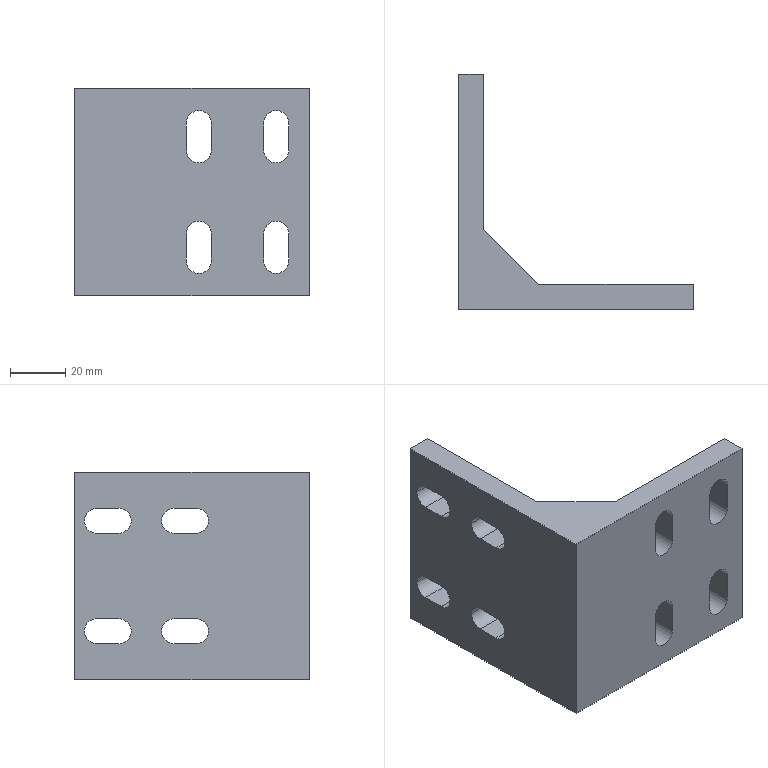Part | 1 solid | 45 faces | box 85 x 85 x 75 mm | volume 113263 mm3 | plane 25 | cylinder 20 | commonest cylinder face diameters 9 x20
STEP:
#1=CARTESIAN_POINT('',(0.,53.5,20.));
#2=VERTEX_POINT('',#1);
#3=CARTESIAN_POINT('',(0.,49.,24.5));
#4=VERTEX_POINT('',#3);
#5=CARTESIAN_POINT('',(0.,49.,20.));
#6=DIRECTION('',(1.,0.,0.));
#7=DIRECTION('',(0.,1.,0.));
#8=AXIS2_PLACEMENT_3D('',#5,#6,#7);
#9=CIRCLE('',#8,4.5);
#10=EDGE_CURVE('',#2,#4,#9,.T.);
#11=ORIENTED_EDGE('',*,*,#10,.F.);
#12=CARTESIAN_POINT('',(9.,53.5,20.));
#13=VERTEX_POINT('',#12);
#14=CARTESIAN_POINT('',(-66.,53.5,20.));
#15=DIRECTION('',(1.,0.,0.));
#16=VECTOR('',#15,1000.);
#17=LINE('',#14,#16);
#18=EDGE_CURVE('',#2,#13,#17,.T.);
#19=ORIENTED_EDGE('',*,*,#18,.T.);
#20=CARTESIAN_POINT('',(9.,49.,24.5));
#21=VERTEX_POINT('',#20);
#22=CARTESIAN_POINT('',(9.,49.,20.));
#23=DIRECTION('',(1.,0.,0.));
#24=DIRECTION('',(0.,-1.,0.));
#25=AXIS2_PLACEMENT_3D('',#22,#23,#24);
#26=CIRCLE('',#25,4.5);
#27=EDGE_CURVE('',#13,#21,#26,.T.);
#28=ORIENTED_EDGE('',*,*,#27,.T.);
#29=CARTESIAN_POINT('',(-66.,49.,24.5));
#30=DIRECTION('',(1.,0.,0.));
#31=VECTOR('',#30,1000.);
#32=LINE('',#29,#31);
#33=EDGE_CURVE('',#4,#21,#32,.T.);
#34=ORIENTED_EDGE('',*,*,#33,.F.);
#35=EDGE_LOOP('',(#11,#19,#28,#34));
#36=FACE_OUTER_BOUND('',#35,.T.);
#37=CARTESIAN_POINT('',(-66.,49.,20.));
#38=DIRECTION('',(1.,0.,0.));
#39=DIRECTION('',(0.,1.,0.));
#40=AXIS2_PLACEMENT_3D('',#37,#38,#39);
#41=CYLINDRICAL_SURFACE('',#40,4.5);
#42=ADVANCED_FACE('',(#36),#41,.F.);
#43=CARTESIAN_POINT('',(0.,53.5,-20.));
#44=VERTEX_POINT('',#43);
#45=CARTESIAN_POINT('',(0.,49.,-15.5));
#46=VERTEX_POINT('',#45);
#47=CARTESIAN_POINT('',(0.,49.,-20.));
#48=DIRECTION('',(1.,0.,0.));
#49=DIRECTION('',(0.,1.,0.));
#50=AXIS2_PLACEMENT_3D('',#47,#48,#49);
#51=CIRCLE('',#50,4.5);
#52=EDGE_CURVE('',#44,#46,#51,.T.);
#53=ORIENTED_EDGE('',*,*,#52,.F.);
#54=CARTESIAN_POINT('',(9.,53.5,-20.));
#55=VERTEX_POINT('',#54);
#56=CARTESIAN_POINT('',(-66.,53.5,-20.));
#57=DIRECTION('',(1.,0.,0.));
#58=VECTOR('',#57,1000.);
#59=LINE('',#56,#58);
#60=EDGE_CURVE('',#44,#55,#59,.T.);
#61=ORIENTED_EDGE('',*,*,#60,.T.);
#62=CARTESIAN_POINT('',(9.,49.,-15.5));
#63=VERTEX_POINT('',#62);
#64=CARTESIAN_POINT('',(9.,49.,-20.));
#65=DIRECTION('',(1.,0.,0.));
#66=DIRECTION('',(0.,1.,0.));
#67=AXIS2_PLACEMENT_3D('',#64,#65,#66);
#68=CIRCLE('',#67,4.5);
#69=EDGE_CURVE('',#55,#63,#68,.T.);
#70=ORIENTED_EDGE('',*,*,#69,.T.);
#71=CARTESIAN_POINT('',(-66.,49.,-15.5));
#72=DIRECTION('',(1.,0.,0.));
#73=VECTOR('',#72,1000.);
#74=LINE('',#71,#73);
#75=EDGE_CURVE('',#46,#63,#74,.T.);
#76=ORIENTED_EDGE('',*,*,#75,.F.);
#77=EDGE_LOOP('',(#53,#61,#70,#76));
#78=FACE_OUTER_BOUND('',#77,.T.);
#79=CARTESIAN_POINT('',(-66.,49.,-20.));
#80=DIRECTION('',(1.,0.,0.));
#81=DIRECTION('',(0.,1.,0.));
#82=AXIS2_PLACEMENT_3D('',#79,#80,#81);
#83=CYLINDRICAL_SURFACE('',#82,4.5);
#84=ADVANCED_FACE('',(#78),#83,.F.);
#85=CARTESIAN_POINT('',(0.,81.5,-20.));
#86=VERTEX_POINT('',#85);
#87=CARTESIAN_POINT('',(0.,77.,-15.5));
#88=VERTEX_POINT('',#87);
#89=CARTESIAN_POINT('',(0.,77.,-20.));
#90=DIRECTION('',(1.,0.,0.));
#91=DIRECTION('',(0.,1.,0.));
#92=AXIS2_PLACEMENT_3D('',#89,#90,#91);
#93=CIRCLE('',#92,4.5);
#94=EDGE_CURVE('',#86,#88,#93,.T.);
#95=ORIENTED_EDGE('',*,*,#94,.F.);
#96=CARTESIAN_POINT('',(9.,81.5,-20.));
#97=VERTEX_POINT('',#96);
#98=CARTESIAN_POINT('',(-66.,81.5,-20.));
#99=DIRECTION('',(1.,0.,0.));
#100=VECTOR('',#99,1000.);
#101=LINE('',#98,#100);
#102=EDGE_CURVE('',#86,#97,#101,.T.);
#103=ORIENTED_EDGE('',*,*,#102,.T.);
#104=CARTESIAN_POINT('',(9.,77.,-15.5));
#105=VERTEX_POINT('',#104);
#106=CARTESIAN_POINT('',(9.,77.,-20.));
#107=DIRECTION('',(1.,0.,0.));
#108=DIRECTION('',(0.,-1.,0.));
#109=AXIS2_PLACEMENT_3D('',#106,#107,#108);
#110=CIRCLE('',#109,4.5);
#111=EDGE_CURVE('',#97,#105,#110,.T.);
#112=ORIENTED_EDGE('',*,*,#111,.T.);
#113=CARTESIAN_POINT('',(-66.,77.,-15.5));
#114=DIRECTION('',(1.,0.,0.));
#115=VECTOR('',#114,1000.);
#116=LINE('',#113,#115);
#117=EDGE_CURVE('',#88,#105,#116,.T.);
#118=ORIENTED_EDGE('',*,*,#117,.F.);
#119=EDGE_LOOP('',(#95,#103,#112,#118));
#120=FACE_OUTER_BOUND('',#119,.T.);
#121=CARTESIAN_POINT('',(-66.,77.,-20.));
#122=DIRECTION('',(1.,0.,0.));
#123=DIRECTION('',(0.,1.,0.));
#124=AXIS2_PLACEMENT_3D('',#121,#122,#123);
#125=CYLINDRICAL_SURFACE('',#124,4.5);
#126=ADVANCED_FACE('',(#120),#125,.F.);
#127=CARTESIAN_POINT('',(0.,81.5,20.));
#128=VERTEX_POINT('',#127);
#129=CARTESIAN_POINT('',(0.,77.,24.5));
#130=VERTEX_POINT('',#129);
#131=CARTESIAN_POINT('',(0.,77.,20.));
#132=DIRECTION('',(1.,0.,0.));
#133=DIRECTION('',(0.,1.,0.));
#134=AXIS2_PLACEMENT_3D('',#131,#132,#133);
#135=CIRCLE('',#134,4.5);
#136=EDGE_CURVE('',#128,#130,#135,.T.);
#137=ORIENTED_EDGE('',*,*,#136,.F.);
#138=CARTESIAN_POINT('',(9.,81.5,20.));
#139=VERTEX_POINT('',#138);
#140=CARTESIAN_POINT('',(-66.,81.5,20.));
#141=DIRECTION('',(1.,0.,0.));
#142=VECTOR('',#141,1000.);
#143=LINE('',#140,#142);
#144=EDGE_CURVE('',#128,#139,#143,.T.);
#145=ORIENTED_EDGE('',*,*,#144,.T.);
#146=CARTESIAN_POINT('',(9.,77.,24.5));
#147=VERTEX_POINT('',#146);
#148=CARTESIAN_POINT('',(9.,77.,20.));
#149=DIRECTION('',(1.,0.,0.));
#150=DIRECTION('',(0.,1.,0.));
#151=AXIS2_PLACEMENT_3D('',#148,#149,#150);
#152=CIRCLE('',#151,4.5);
#153=EDGE_CURVE('',#139,#147,#152,.T.);
#154=ORIENTED_EDGE('',*,*,#153,.T.);
#155=CARTESIAN_POINT('',(-66.,77.,24.5));
#156=DIRECTION('',(1.,0.,0.));
#157=VECTOR('',#156,1000.);
#158=LINE('',#155,#157);
#159=EDGE_CURVE('',#130,#147,#158,.T.);
#160=ORIENTED_EDGE('',*,*,#159,.F.);
#161=EDGE_LOOP('',(#137,#145,#154,#160));
#162=FACE_OUTER_BOUND('',#161,.T.);
#163=CARTESIAN_POINT('',(-66.,77.,20.));
#164=DIRECTION('',(1.,0.,0.));
#165=DIRECTION('',(0.,1.,0.));
#166=AXIS2_PLACEMENT_3D('',#163,#164,#165);
#167=CYLINDRICAL_SURFACE('',#166,4.5);
#168=ADVANCED_FACE('',(#162),#167,.F.);
#169=CARTESIAN_POINT('',(0.,41.,24.5));
#170=VERTEX_POINT('',#169);
#171=CARTESIAN_POINT('',(0.,85.,24.5));
#172=DIRECTION('',(0.,-1.,0.));
#173=VECTOR('',#172,1000.);
#174=LINE('',#171,#173);
#175=EDGE_CURVE('',#4,#170,#174,.T.);
#176=ORIENTED_EDGE('',*,*,#175,.T.);
#177=CARTESIAN_POINT('',(0.,41.,15.5));
#178=VERTEX_POINT('',#177);
#179=CARTESIAN_POINT('',(0.,41.,20.));
#180=DIRECTION('',(1.,0.,0.));
#181=DIRECTION('',(0.,1.,0.));
#182=AXIS2_PLACEMENT_3D('',#179,#180,#181);
#183=CIRCLE('',#182,4.5);
#184=EDGE_CURVE('',#170,#178,#183,.T.);
#185=ORIENTED_EDGE('',*,*,#184,.T.);
#186=CARTESIAN_POINT('',(0.,49.,15.5));
#187=VERTEX_POINT('',#186);
#188=CARTESIAN_POINT('',(0.,85.,15.5));
#189=DIRECTION('',(0.,1.,0.));
#190=VECTOR('',#189,1000.);
#191=LINE('',#188,#190);
#192=EDGE_CURVE('',#178,#187,#191,.T.);
#193=ORIENTED_EDGE('',*,*,#192,.T.);
#194=CARTESIAN_POINT('',(0.,49.,20.));
#195=DIRECTION('',(1.,0.,0.));
#196=DIRECTION('',(0.,1.,0.));
#197=AXIS2_PLACEMENT_3D('',#194,#195,#196);
#198=CIRCLE('',#197,4.5);
#199=EDGE_CURVE('',#187,#2,#198,.T.);
#200=ORIENTED_EDGE('',*,*,#199,.T.);
#201=ORIENTED_EDGE('',*,*,#10,.T.);
#202=EDGE_LOOP('',(#176,#185,#193,#200,#201));
#203=FACE_BOUND('',#202,.T.);
#204=CARTESIAN_POINT('',(0.,41.,-15.5));
#205=VERTEX_POINT('',#204);
#206=CARTESIAN_POINT('',(0.,85.,-15.5));
#207=DIRECTION('',(0.,-1.,0.));
#208=VECTOR('',#207,1000.);
#209=LINE('',#206,#208);
#210=EDGE_CURVE('',#46,#205,#209,.T.);
#211=ORIENTED_EDGE('',*,*,#210,.T.);
#212=CARTESIAN_POINT('',(0.,41.,-24.5));
#213=VERTEX_POINT('',#212);
#214=CARTESIAN_POINT('',(0.,41.,-20.));
#215=DIRECTION('',(1.,0.,0.));
#216=DIRECTION('',(0.,1.,0.));
#217=AXIS2_PLACEMENT_3D('',#214,#215,#216);
#218=CIRCLE('',#217,4.5);
#219=EDGE_CURVE('',#205,#213,#218,.T.);
#220=ORIENTED_EDGE('',*,*,#219,.T.);
#221=CARTESIAN_POINT('',(0.,49.,-24.5));
#222=VERTEX_POINT('',#221);
#223=CARTESIAN_POINT('',(0.,85.,-24.5));
#224=DIRECTION('',(0.,1.,0.));
#225=VECTOR('',#224,1000.);
#226=LINE('',#223,#225);
#227=EDGE_CURVE('',#213,#222,#226,.T.);
#228=ORIENTED_EDGE('',*,*,#227,.T.);
#229=CARTESIAN_POINT('',(0.,49.,-20.));
#230=DIRECTION('',(1.,0.,0.));
#231=DIRECTION('',(0.,1.,0.));
#232=AXIS2_PLACEMENT_3D('',#229,#230,#231);
#233=CIRCLE('',#232,4.5);
#234=EDGE_CURVE('',#222,#44,#233,.T.);
#235=ORIENTED_EDGE('',*,*,#234,.T.);
#236=ORIENTED_EDGE('',*,*,#52,.T.);
#237=EDGE_LOOP('',(#211,#220,#228,#235,#236));
#238=FACE_BOUND('',#237,.T.);
#239=CARTESIAN_POINT('',(0.,69.,-24.5));
#240=VERTEX_POINT('',#239);
#241=CARTESIAN_POINT('',(0.,77.,-24.5));
#242=VERTEX_POINT('',#241);
#243=CARTESIAN_POINT('',(0.,85.,-24.5));
#244=DIRECTION('',(0.,1.,0.));
#245=VECTOR('',#244,1000.);
#246=LINE('',#243,#245);
#247=EDGE_CURVE('',#240,#242,#246,.T.);
#248=ORIENTED_EDGE('',*,*,#247,.T.);
#249=CARTESIAN_POINT('',(0.,77.,-20.));
#250=DIRECTION('',(1.,0.,0.));
#251=DIRECTION('',(0.,1.,0.));
#252=AXIS2_PLACEMENT_3D('',#249,#250,#251);
#253=CIRCLE('',#252,4.5);
#254=EDGE_CURVE('',#242,#86,#253,.T.);
#255=ORIENTED_EDGE('',*,*,#254,.T.);
#256=ORIENTED_EDGE('',*,*,#94,.T.);
#257=CARTESIAN_POINT('',(0.,69.,-15.5));
#258=VERTEX_POINT('',#257);
#259=CARTESIAN_POINT('',(0.,85.,-15.5));
#260=DIRECTION('',(0.,-1.,0.));
#261=VECTOR('',#260,1000.);
#262=LINE('',#259,#261);
#263=EDGE_CURVE('',#88,#258,#262,.T.);
#264=ORIENTED_EDGE('',*,*,#263,.T.);
#265=CARTESIAN_POINT('',(0.,69.,-20.));
#266=DIRECTION('',(1.,0.,0.));
#267=DIRECTION('',(0.,1.,0.));
#268=AXIS2_PLACEMENT_3D('',#265,#266,#267);
#269=CIRCLE('',#268,4.5);
#270=EDGE_CURVE('',#258,#240,#269,.T.);
#271=ORIENTED_EDGE('',*,*,#270,.T.);
#272=EDGE_LOOP('',(#248,#255,#256,#264,#271));
#273=FACE_BOUND('',#272,.T.);
#274=CARTESIAN_POINT('',(0.,69.,15.5));
#275=VERTEX_POINT('',#274);
#276=CARTESIAN_POINT('',(0.,77.,15.5));
#277=VERTEX_POINT('',#276);
#278=CARTESIAN_POINT('',(0.,85.,15.5));
#279=DIRECTION('',(0.,1.,0.));
#280=VECTOR('',#279,1000.);
#281=LINE('',#278,#280);
#282=EDGE_CURVE('',#275,#277,#281,.T.);
#283=ORIENTED_EDGE('',*,*,#282,.T.);
#284=CARTESIAN_POINT('',(0.,77.,20.));
#285=DIRECTION('',(1.,0.,0.));
#286=DIRECTION('',(0.,1.,0.));
#287=AXIS2_PLACEMENT_3D('',#284,#285,#286);
#288=CIRCLE('',#287,4.5);
#289=EDGE_CURVE('',#277,#128,#288,.T.);
#290=ORIENTED_EDGE('',*,*,#289,.T.);
#291=ORIENTED_EDGE('',*,*,#136,.T.);
#292=CARTESIAN_POINT('',(0.,69.,24.5));
#293=VERTEX_POINT('',#292);
#294=CARTESIAN_POINT('',(0.,85.,24.5));
#295=DIRECTION('',(0.,-1.,0.));
#296=VECTOR('',#295,1000.);
#297=LINE('',#294,#296);
#298=EDGE_CURVE('',#130,#293,#297,.T.);
#299=ORIENTED_EDGE('',*,*,#298,.T.);
#300=CARTESIAN_POINT('',(0.,69.,20.));
#301=DIRECTION('',(1.,0.,0.));
#302=DIRECTION('',(0.,1.,0.));
#303=AXIS2_PLACEMENT_3D('',#300,#301,#302);
#304=CIRCLE('',#303,4.5);
#305=EDGE_CURVE('',#293,#275,#304,.T.);
#306=ORIENTED_EDGE('',*,*,#305,.T.);
#307=EDGE_LOOP('',(#283,#290,#291,#299,#306));
#308=FACE_BOUND('',#307,.T.);
#309=CARTESIAN_POINT('',(0.,85.,-37.5));
#310=VERTEX_POINT('',#309);
#311=CARTESIAN_POINT('',(0.,0.,-37.5));
#312=VERTEX_POINT('',#311);
#313=CARTESIAN_POINT('',(0.,85.,-37.5));
#314=DIRECTION('',(0.,-1.,0.));
#315=VECTOR('',#314,1000.);
#316=LINE('',#313,#315);
#317=EDGE_CURVE('',#310,#312,#316,.T.);
#318=ORIENTED_EDGE('',*,*,#317,.T.);
#319=CARTESIAN_POINT('',(0.,0.,37.5));
#320=VERTEX_POINT('',#319);
#321=CARTESIAN_POINT('',(0.,0.,37.5));
#322=DIRECTION('',(0.,0.,-1.));
#323=VECTOR('',#322,1000.);
#324=LINE('',#321,#323);
#325=EDGE_CURVE('',#320,#312,#324,.T.);
#326=ORIENTED_EDGE('',*,*,#325,.F.);
#327=CARTESIAN_POINT('',(0.,85.,37.5));
#328=VERTEX_POINT('',#327);
#329=CARTESIAN_POINT('',(0.,85.,37.5));
#330=DIRECTION('',(0.,-1.,0.));
#331=VECTOR('',#330,1000.);
#332=LINE('',#329,#331);
#333=EDGE_CURVE('',#328,#320,#332,.T.);
#334=ORIENTED_EDGE('',*,*,#333,.F.);
#335=CARTESIAN_POINT('',(0.,85.,37.5));
#336=DIRECTION('',(0.,0.,-1.));
#337=VECTOR('',#336,1000.);
#338=LINE('',#335,#337);
#339=EDGE_CURVE('',#328,#310,#338,.T.);
#340=ORIENTED_EDGE('',*,*,#339,.T.);
#341=EDGE_LOOP('',(#318,#326,#334,#340));
#342=FACE_OUTER_BOUND('',#341,.T.);
#343=CARTESIAN_POINT('',(0.,85.,37.5));
#344=DIRECTION('',(1.,0.,0.));
#345=DIRECTION('',(0.,1.,0.));
#346=AXIS2_PLACEMENT_3D('',#343,#344,#345);
#347=PLANE('',#346);
#348=ADVANCED_FACE('',(#203,#238,#273,#308,#342),#347,.F.);
#349=CARTESIAN_POINT('',(68.5,0.,15.));
#350=VERTEX_POINT('',#349);
#351=CARTESIAN_POINT('',(68.5,0.,25.));
#352=VERTEX_POINT('',#351);
#353=CARTESIAN_POINT('',(68.5,0.,37.5));
#354=DIRECTION('',(0.,0.,1.));
#355=VECTOR('',#354,1000.);
#356=LINE('',#353,#355);
#357=EDGE_CURVE('',#350,#352,#356,.T.);
#358=ORIENTED_EDGE('',*,*,#357,.T.);
#359=CARTESIAN_POINT('',(77.5,0.,25.));
#360=VERTEX_POINT('',#359);
#361=CARTESIAN_POINT('',(73.,0.,25.));
#362=DIRECTION('',(0.,1.,0.));
#363=DIRECTION('',(0.,0.,1.));
#364=AXIS2_PLACEMENT_3D('',#361,#362,#363);
#365=CIRCLE('',#364,4.5);
#366=EDGE_CURVE('',#352,#360,#365,.T.);
#367=ORIENTED_EDGE('',*,*,#366,.T.);
#368=CARTESIAN_POINT('',(77.5,0.,15.));
#369=VERTEX_POINT('',#368);
#370=CARTESIAN_POINT('',(77.5,0.,37.5));
#371=DIRECTION('',(0.,0.,-1.));
#372=VECTOR('',#371,1000.);
#373=LINE('',#370,#372);
#374=EDGE_CURVE('',#360,#369,#373,.T.);
#375=ORIENTED_EDGE('',*,*,#374,.T.);
#376=CARTESIAN_POINT('',(73.,0.,15.));
#377=DIRECTION('',(0.,1.,0.));
#378=DIRECTION('',(0.,0.,1.));
#379=AXIS2_PLACEMENT_3D('',#376,#377,#378);
#380=CIRCLE('',#379,4.5);
#381=EDGE_CURVE('',#369,#350,#380,.T.);
#382=ORIENTED_EDGE('',*,*,#381,.T.);
#383=EDGE_LOOP('',(#358,#367,#375,#382));
#384=FACE_BOUND('',#383,.T.);
#385=CARTESIAN_POINT('',(40.5,0.,15.));
#386=VERTEX_POINT('',#385);
#387=CARTESIAN_POINT('',(40.5,0.,25.));
#388=VERTEX_POINT('',#387);
#389=CARTESIAN_POINT('',(40.5,0.,37.5));
#390=DIRECTION('',(0.,0.,1.));
#391=VECTOR('',#390,1000.);
#392=LINE('',#389,#391);
#393=EDGE_CURVE('',#386,#388,#392,.T.);
#394=ORIENTED_EDGE('',*,*,#393,.T.);
#395=CARTESIAN_POINT('',(49.5,0.,25.));
#396=VERTEX_POINT('',#395);
#397=CARTESIAN_POINT('',(45.,0.,25.));
#398=DIRECTION('',(0.,1.,0.));
#399=DIRECTION('',(0.,0.,1.));
#400=AXIS2_PLACEMENT_3D('',#397,#398,#399);
#401=CIRCLE('',#400,4.5);
#402=EDGE_CURVE('',#388,#396,#401,.T.);
#403=ORIENTED_EDGE('',*,*,#402,.T.);
#404=CARTESIAN_POINT('',(49.5,0.,15.));
#405=VERTEX_POINT('',#404);
#406=CARTESIAN_POINT('',(49.5,0.,37.5));
#407=DIRECTION('',(0.,0.,-1.));
#408=VECTOR('',#407,1000.);
#409=LINE('',#406,#408);
#410=EDGE_CURVE('',#396,#405,#409,.T.);
#411=ORIENTED_EDGE('',*,*,#410,.T.);
#412=CARTESIAN_POINT('',(45.,0.,15.));
#413=DIRECTION('',(0.,1.,0.));
#414=DIRECTION('',(0.,0.,1.));
#415=AXIS2_PLACEMENT_3D('',#412,#413,#414);
#416=CIRCLE('',#415,4.5);
#417=EDGE_CURVE('',#405,#386,#416,.T.);
#418=ORIENTED_EDGE('',*,*,#417,.T.);
#419=EDGE_LOOP('',(#394,#403,#411,#418));
#420=FACE_BOUND('',#419,.T.);
#421=CARTESIAN_POINT('',(68.5,0.,-25.));
#422=VERTEX_POINT('',#421);
#423=CARTESIAN_POINT('',(68.5,0.,-15.));
#424=VERTEX_POINT('',#423);
#425=CARTESIAN_POINT('',(68.5,0.,37.5));
#426=DIRECTION('',(0.,0.,1.));
#427=VECTOR('',#426,1000.);
#428=LINE('',#425,#427);
#429=EDGE_CURVE('',#422,#424,#428,.T.);
#430=ORIENTED_EDGE('',*,*,#429,.T.);
#431=CARTESIAN_POINT('',(77.5,0.,-15.));
#432=VERTEX_POINT('',#431);
#433=CARTESIAN_POINT('',(73.,0.,-15.));
#434=DIRECTION('',(0.,1.,0.));
#435=DIRECTION('',(0.,0.,1.));
#436=AXIS2_PLACEMENT_3D('',#433,#434,#435);
#437=CIRCLE('',#436,4.5);
#438=EDGE_CURVE('',#424,#432,#437,.T.);
#439=ORIENTED_EDGE('',*,*,#438,.T.);
#440=CARTESIAN_POINT('',(77.5,0.,-25.));
#441=VERTEX_POINT('',#440);
#442=CARTESIAN_POINT('',(77.5,0.,37.5));
#443=DIRECTION('',(0.,0.,-1.));
#444=VECTOR('',#443,1000.);
#445=LINE('',#442,#444);
#446=EDGE_CURVE('',#432,#441,#445,.T.);
#447=ORIENTED_EDGE('',*,*,#446,.T.);
#448=CARTESIAN_POINT('',(73.,0.,-25.));
#449=DIRECTION('',(0.,1.,0.));
#450=DIRECTION('',(0.,0.,1.));
#451=AXIS2_PLACEMENT_3D('',#448,#449,#450);
#452=CIRCLE('',#451,4.5);
#453=EDGE_CURVE('',#441,#422,#452,.T.);
#454=ORIENTED_EDGE('',*,*,#453,.T.);
#455=EDGE_LOOP('',(#430,#439,#447,#454));
#456=FACE_BOUND('',#455,.T.);
#457=CARTESIAN_POINT('',(40.5,0.,-25.));
#458=VERTEX_POINT('',#457);
#459=CARTESIAN_POINT('',(40.5,0.,-15.));
#460=VERTEX_POINT('',#459);
#461=CARTESIAN_POINT('',(40.5,0.,37.5));
#462=DIRECTION('',(0.,0.,1.));
#463=VECTOR('',#462,1000.);
#464=LINE('',#461,#463);
#465=EDGE_CURVE('',#458,#460,#464,.T.);
#466=ORIENTED_EDGE('',*,*,#465,.T.);
#467=CARTESIAN_POINT('',(49.5,0.,-15.));
#468=VERTEX_POINT('',#467);
#469=CARTESIAN_POINT('',(45.,0.,-15.));
#470=DIRECTION('',(0.,1.,0.));
#471=DIRECTION('',(0.,0.,1.));
#472=AXIS2_PLACEMENT_3D('',#469,#470,#471);
#473=CIRCLE('',#472,4.5);
#474=EDGE_CURVE('',#460,#468,#473,.T.);
#475=ORIENTED_EDGE('',*,*,#474,.T.);
#476=CARTESIAN_POINT('',(49.5,0.,-25.));
#477=VERTEX_POINT('',#476);
#478=CARTESIAN_POINT('',(49.5,0.,37.5));
#479=DIRECTION('',(0.,0.,-1.));
#480=VECTOR('',#479,1000.);
#481=LINE('',#478,#480);
#482=EDGE_CURVE('',#468,#477,#481,.T.);
#483=ORIENTED_EDGE('',*,*,#482,.T.);
#484=CARTESIAN_POINT('',(45.,0.,-25.));
#485=DIRECTION('',(0.,1.,0.));
#486=DIRECTION('',(0.,0.,1.));
#487=AXIS2_PLACEMENT_3D('',#484,#485,#486);
#488=CIRCLE('',#487,4.5);
#489=EDGE_CURVE('',#477,#458,#488,.T.);
#490=ORIENTED_EDGE('',*,*,#489,.T.);
#491=EDGE_LOOP('',(#466,#475,#483,#490));
#492=FACE_BOUND('',#491,.T.);
#493=CARTESIAN_POINT('',(85.,0.,-37.5));
#494=VERTEX_POINT('',#493);
#495=CARTESIAN_POINT('',(0.,0.,-37.5));
#496=DIRECTION('',(1.,0.,0.));
#497=VECTOR('',#496,1000.);
#498=LINE('',#495,#497);
#499=EDGE_CURVE('',#312,#494,#498,.T.);
#500=ORIENTED_EDGE('',*,*,#499,.T.);
#501=CARTESIAN_POINT('',(85.,0.,37.5));
#502=VERTEX_POINT('',#501);
#503=CARTESIAN_POINT('',(85.,0.,37.5));
#504=DIRECTION('',(0.,0.,-1.));
#505=VECTOR('',#504,1000.);
#506=LINE('',#503,#505);
#507=EDGE_CURVE('',#502,#494,#506,.T.);
#508=ORIENTED_EDGE('',*,*,#507,.F.);
#509=CARTESIAN_POINT('',(0.,0.,37.5));
#510=DIRECTION('',(1.,0.,0.));
#511=VECTOR('',#510,1000.);
#512=LINE('',#509,#511);
#513=EDGE_CURVE('',#320,#502,#512,.T.);
#514=ORIENTED_EDGE('',*,*,#513,.F.);
#515=ORIENTED_EDGE('',*,*,#325,.T.);
#516=EDGE_LOOP('',(#500,#508,#514,#515));
#517=FACE_OUTER_BOUND('',#516,.T.);
#518=CARTESIAN_POINT('',(0.,0.,37.5));
#519=DIRECTION('',(0.,1.,0.));
#520=DIRECTION('',(0.,0.,1.));
#521=AXIS2_PLACEMENT_3D('',#518,#519,#520);
#522=PLANE('',#521);
#523=ADVANCED_FACE('',(#384,#420,#456,#492,#517),#522,.F.);
#524=CARTESIAN_POINT('',(85.,9.,-37.5));
#525=VERTEX_POINT('',#524);
#526=CARTESIAN_POINT('',(85.,0.,-37.5));
#527=DIRECTION('',(0.,1.,0.));
#528=VECTOR('',#527,1000.);
#529=LINE('',#526,#528);
#530=EDGE_CURVE('',#494,#525,#529,.T.);
#531=ORIENTED_EDGE('',*,*,#530,.T.);
#532=CARTESIAN_POINT('',(85.,9.,37.5));
#533=VERTEX_POINT('',#532);
#534=CARTESIAN_POINT('',(85.,9.,37.5));
#535=DIRECTION('',(0.,0.,-1.));
#536=VECTOR('',#535,1000.);
#537=LINE('',#534,#536);
#538=EDGE_CURVE('',#533,#525,#537,.T.);
#539=ORIENTED_EDGE('',*,*,#538,.F.);
#540=CARTESIAN_POINT('',(85.,0.,37.5));
#541=DIRECTION('',(0.,1.,0.));
#542=VECTOR('',#541,1000.);
#543=LINE('',#540,#542);
#544=EDGE_CURVE('',#502,#533,#543,.T.);
#545=ORIENTED_EDGE('',*,*,#544,.F.);
#546=ORIENTED_EDGE('',*,*,#507,.T.);
#547=EDGE_LOOP('',(#531,#539,#545,#546));
#548=FACE_OUTER_BOUND('',#547,.T.);
#549=CARTESIAN_POINT('',(85.,0.,37.5));
#550=DIRECTION('',(-1.,0.,0.));
#551=DIRECTION('',(0.,0.,1.));
#552=AXIS2_PLACEMENT_3D('',#549,#550,#551);
#553=PLANE('',#552);
#554=ADVANCED_FACE('',(#548),#553,.F.);
#555=CARTESIAN_POINT('',(77.5,9.,25.));
#556=VERTEX_POINT('',#555);
#557=CARTESIAN_POINT('',(77.5,9.,15.));
#558=VERTEX_POINT('',#557);
#559=CARTESIAN_POINT('',(77.5,9.,25.));
#560=DIRECTION('',(0.,0.,-1.));
#561=VECTOR('',#560,1000.);
#562=LINE('',#559,#561);
#563=EDGE_CURVE('',#556,#558,#562,.T.);
#564=ORIENTED_EDGE('',*,*,#563,.F.);
#565=CARTESIAN_POINT('',(68.5,9.,25.));
#566=VERTEX_POINT('',#565);
#567=CARTESIAN_POINT('',(73.,9.,25.));
#568=DIRECTION('',(0.,1.,0.));
#569=DIRECTION('',(-1.,0.,0.));
#570=AXIS2_PLACEMENT_3D('',#567,#568,#569);
#571=CIRCLE('',#570,4.5);
#572=EDGE_CURVE('',#566,#556,#571,.T.);
#573=ORIENTED_EDGE('',*,*,#572,.F.);
#574=CARTESIAN_POINT('',(68.5,9.,15.));
#575=VERTEX_POINT('',#574);
#576=CARTESIAN_POINT('',(68.5,9.,25.));
#577=DIRECTION('',(0.,0.,1.));
#578=VECTOR('',#577,1000.);
#579=LINE('',#576,#578);
#580=EDGE_CURVE('',#575,#566,#579,.T.);
#581=ORIENTED_EDGE('',*,*,#580,.F.);
#582=CARTESIAN_POINT('',(73.,9.,15.));
#583=DIRECTION('',(0.,1.,0.));
#584=DIRECTION('',(-1.,0.,0.));
#585=AXIS2_PLACEMENT_3D('',#582,#583,#584);
#586=CIRCLE('',#585,4.5);
#587=EDGE_CURVE('',#558,#575,#586,.T.);
#588=ORIENTED_EDGE('',*,*,#587,.F.);
#589=EDGE_LOOP('',(#564,#573,#581,#588));
#590=FACE_BOUND('',#589,.T.);
#591=CARTESIAN_POINT('',(49.5,9.,25.));
#592=VERTEX_POINT('',#591);
#593=CARTESIAN_POINT('',(49.5,9.,15.));
#594=VERTEX_POINT('',#593);
#595=CARTESIAN_POINT('',(49.5,9.,25.));
#596=DIRECTION('',(0.,0.,-1.));
#597=VECTOR('',#596,1000.);
#598=LINE('',#595,#597);
#599=EDGE_CURVE('',#592,#594,#598,.T.);
#600=ORIENTED_EDGE('',*,*,#599,.F.);
#601=CARTESIAN_POINT('',(40.5,9.,25.));
#602=VERTEX_POINT('',#601);
#603=CARTESIAN_POINT('',(45.,9.,25.));
#604=DIRECTION('',(0.,1.,0.));
#605=DIRECTION('',(-1.,0.,0.));
#606=AXIS2_PLACEMENT_3D('',#603,#604,#605);
#607=CIRCLE('',#606,4.5);
#608=EDGE_CURVE('',#602,#592,#607,.T.);
#609=ORIENTED_EDGE('',*,*,#608,.F.);
#610=CARTESIAN_POINT('',(40.5,9.,15.));
#611=VERTEX_POINT('',#610);
#612=CARTESIAN_POINT('',(40.5,9.,25.));
#613=DIRECTION('',(0.,0.,1.));
#614=VECTOR('',#613,1000.);
#615=LINE('',#612,#614);
#616=EDGE_CURVE('',#611,#602,#615,.T.);
#617=ORIENTED_EDGE('',*,*,#616,.F.);
#618=CARTESIAN_POINT('',(45.,9.,15.));
#619=DIRECTION('',(0.,1.,0.));
#620=DIRECTION('',(-1.,0.,0.));
#621=AXIS2_PLACEMENT_3D('',#618,#619,#620);
#622=CIRCLE('',#621,4.5);
#623=EDGE_CURVE('',#594,#611,#622,.T.);
#624=ORIENTED_EDGE('',*,*,#623,.F.);
#625=EDGE_LOOP('',(#600,#609,#617,#624));
#626=FACE_BOUND('',#625,.T.);
#627=CARTESIAN_POINT('',(77.5,9.,-15.));
#628=VERTEX_POINT('',#627);
#629=CARTESIAN_POINT('',(77.5,9.,-25.));
#630=VERTEX_POINT('',#629);
#631=CARTESIAN_POINT('',(77.5,9.,-15.));
#632=DIRECTION('',(0.,0.,-1.));
#633=VECTOR('',#632,1000.);
#634=LINE('',#631,#633);
#635=EDGE_CURVE('',#628,#630,#634,.T.);
#636=ORIENTED_EDGE('',*,*,#635,.F.);
#637=CARTESIAN_POINT('',(68.5,9.,-15.));
#638=VERTEX_POINT('',#637);
#639=CARTESIAN_POINT('',(73.,9.,-15.));
#640=DIRECTION('',(0.,1.,0.));
#641=DIRECTION('',(-1.,0.,0.));
#642=AXIS2_PLACEMENT_3D('',#639,#640,#641);
#643=CIRCLE('',#642,4.5);
#644=EDGE_CURVE('',#638,#628,#643,.T.);
#645=ORIENTED_EDGE('',*,*,#644,.F.);
#646=CARTESIAN_POINT('',(68.5,9.,-25.));
#647=VERTEX_POINT('',#646);
#648=CARTESIAN_POINT('',(68.5,9.,-15.));
#649=DIRECTION('',(0.,0.,1.));
#650=VECTOR('',#649,1000.);
#651=LINE('',#648,#650);
#652=EDGE_CURVE('',#647,#638,#651,.T.);
#653=ORIENTED_EDGE('',*,*,#652,.F.);
#654=CARTESIAN_POINT('',(73.,9.,-25.));
#655=DIRECTION('',(0.,1.,0.));
#656=DIRECTION('',(-1.,0.,0.));
#657=AXIS2_PLACEMENT_3D('',#654,#655,#656);
#658=CIRCLE('',#657,4.5);
#659=EDGE_CURVE('',#630,#647,#658,.T.);
#660=ORIENTED_EDGE('',*,*,#659,.F.);
#661=EDGE_LOOP('',(#636,#645,#653,#660));
#662=FACE_BOUND('',#661,.T.);
#663=CARTESIAN_POINT('',(49.5,9.,-15.));
#664=VERTEX_POINT('',#663);
#665=CARTESIAN_POINT('',(49.5,9.,-25.));
#666=VERTEX_POINT('',#665);
#667=CARTESIAN_POINT('',(49.5,9.,-15.));
#668=DIRECTION('',(0.,0.,-1.));
#669=VECTOR('',#668,1000.);
#670=LINE('',#667,#669);
#671=EDGE_CURVE('',#664,#666,#670,.T.);
#672=ORIENTED_EDGE('',*,*,#671,.F.);
#673=CARTESIAN_POINT('',(40.5,9.,-15.));
#674=VERTEX_POINT('',#673);
#675=CARTESIAN_POINT('',(45.,9.,-15.));
#676=DIRECTION('',(0.,1.,0.));
#677=DIRECTION('',(-1.,0.,0.));
#678=AXIS2_PLACEMENT_3D('',#675,#676,#677);
#679=CIRCLE('',#678,4.5);
#680=EDGE_CURVE('',#674,#664,#679,.T.);
#681=ORIENTED_EDGE('',*,*,#680,.F.);
#682=CARTESIAN_POINT('',(40.5,9.,-25.));
#683=VERTEX_POINT('',#682);
#684=CARTESIAN_POINT('',(40.5,9.,-15.));
#685=DIRECTION('',(0.,0.,1.));
#686=VECTOR('',#685,1000.);
#687=LINE('',#684,#686);
#688=EDGE_CURVE('',#683,#674,#687,.T.);
#689=ORIENTED_EDGE('',*,*,#688,.F.);
#690=CARTESIAN_POINT('',(45.,9.,-25.));
#691=DIRECTION('',(0.,1.,0.));
#692=DIRECTION('',(-1.,0.,0.));
#693=AXIS2_PLACEMENT_3D('',#690,#691,#692);
#694=CIRCLE('',#693,4.5);
#695=EDGE_CURVE('',#666,#683,#694,.T.);
#696=ORIENTED_EDGE('',*,*,#695,.F.);
#697=EDGE_LOOP('',(#672,#681,#689,#696));
#698=FACE_BOUND('',#697,.T.);
#699=CARTESIAN_POINT('',(29.,9.,-37.5));
#700=VERTEX_POINT('',#699);
#701=CARTESIAN_POINT('',(85.,9.,-37.5));
#702=DIRECTION('',(-1.,0.,0.));
#703=VECTOR('',#702,1000.);
#704=LINE('',#701,#703);
#705=EDGE_CURVE('',#525,#700,#704,.T.);
#706=ORIENTED_EDGE('',*,*,#705,.T.);
#707=CARTESIAN_POINT('',(29.,9.,37.5));
#708=VERTEX_POINT('',#707);
#709=CARTESIAN_POINT('',(29.,9.,37.5));
#710=DIRECTION('',(0.,0.,-1.));
#711=VECTOR('',#710,1000.);
#712=LINE('',#709,#711);
#713=EDGE_CURVE('',#708,#700,#712,.T.);
#714=ORIENTED_EDGE('',*,*,#713,.F.);
#715=CARTESIAN_POINT('',(85.,9.,37.5));
#716=DIRECTION('',(-1.,0.,0.));
#717=VECTOR('',#716,1000.);
#718=LINE('',#715,#717);
#719=EDGE_CURVE('',#533,#708,#718,.T.);
#720=ORIENTED_EDGE('',*,*,#719,.F.);
#721=ORIENTED_EDGE('',*,*,#538,.T.);
#722=EDGE_LOOP('',(#706,#714,#720,#721));
#723=FACE_OUTER_BOUND('',#722,.T.);
#724=CARTESIAN_POINT('',(85.,9.,37.5));
#725=DIRECTION('',(0.,-1.,0.));
#726=DIRECTION('',(1.,0.,0.));
#727=AXIS2_PLACEMENT_3D('',#724,#725,#726);
#728=PLANE('',#727);
#729=ADVANCED_FACE('',(#590,#626,#662,#698,#723),#728,.F.);
#730=CARTESIAN_POINT('',(9.,29.,-37.5));
#731=VERTEX_POINT('',#730);
#732=CARTESIAN_POINT('',(9.,29.,-37.5));
#733=DIRECTION('',(-0.7071,0.7071,0.));
#734=VECTOR('',#733,1000.);
#735=LINE('',#732,#734);
#736=EDGE_CURVE('',#700,#731,#735,.T.);
#737=ORIENTED_EDGE('',*,*,#736,.T.);
#738=CARTESIAN_POINT('',(9.,29.,37.5));
#739=VERTEX_POINT('',#738);
#740=CARTESIAN_POINT('',(9.,29.,37.5));
#741=DIRECTION('',(0.,0.,-1.));
#742=VECTOR('',#741,1000.);
#743=LINE('',#740,#742);
#744=EDGE_CURVE('',#739,#731,#743,.T.);
#745=ORIENTED_EDGE('',*,*,#744,.F.);
#746=CARTESIAN_POINT('',(9.,29.,37.5));
#747=DIRECTION('',(-0.7071,0.7071,0.));
#748=VECTOR('',#747,1000.);
#749=LINE('',#746,#748);
#750=EDGE_CURVE('',#708,#739,#749,.T.);
#751=ORIENTED_EDGE('',*,*,#750,.F.);
#752=ORIENTED_EDGE('',*,*,#713,.T.);
#753=EDGE_LOOP('',(#737,#745,#751,#752));
#754=FACE_OUTER_BOUND('',#753,.T.);
#755=CARTESIAN_POINT('',(9.,29.,37.5));
#756=DIRECTION('',(-0.7071,-0.7071,0.));
#757=DIRECTION('',(0.7071,-0.7071,0.));
#758=AXIS2_PLACEMENT_3D('',#755,#756,#757);
#759=PLANE('',#758);
#760=ADVANCED_FACE('',(#754),#759,.F.);
#761=CARTESIAN_POINT('',(9.,41.,15.5));
#762=VERTEX_POINT('',#761);
#763=CARTESIAN_POINT('',(9.,49.,15.5));
#764=VERTEX_POINT('',#763);
#765=CARTESIAN_POINT('',(9.,41.,15.5));
#766=DIRECTION('',(0.,1.,0.));
#767=VECTOR('',#766,1000.);
#768=LINE('',#765,#767);
#769=EDGE_CURVE('',#762,#764,#768,.T.);
#770=ORIENTED_EDGE('',*,*,#769,.F.);
#771=CARTESIAN_POINT('',(9.,41.,24.5));
#772=VERTEX_POINT('',#771);
#773=CARTESIAN_POINT('',(9.,41.,20.));
#774=DIRECTION('',(1.,0.,0.));
#775=DIRECTION('',(0.,-1.,0.));
#776=AXIS2_PLACEMENT_3D('',#773,#774,#775);
#777=CIRCLE('',#776,4.5);
#778=EDGE_CURVE('',#772,#762,#777,.T.);
#779=ORIENTED_EDGE('',*,*,#778,.F.);
#780=CARTESIAN_POINT('',(9.,41.,24.5));
#781=DIRECTION('',(0.,-1.,0.));
#782=VECTOR('',#781,1000.);
#783=LINE('',#780,#782);
#784=EDGE_CURVE('',#21,#772,#783,.T.);
#785=ORIENTED_EDGE('',*,*,#784,.F.);
#786=ORIENTED_EDGE('',*,*,#27,.F.);
#787=CARTESIAN_POINT('',(9.,49.,20.));
#788=DIRECTION('',(1.,0.,0.));
#789=DIRECTION('',(0.,-1.,0.));
#790=AXIS2_PLACEMENT_3D('',#787,#788,#789);
#791=CIRCLE('',#790,4.5);
#792=EDGE_CURVE('',#764,#13,#791,.T.);
#793=ORIENTED_EDGE('',*,*,#792,.F.);
#794=EDGE_LOOP('',(#770,#779,#785,#786,#793));
#795=FACE_BOUND('',#794,.T.);
#796=CARTESIAN_POINT('',(9.,41.,-24.5));
#797=VERTEX_POINT('',#796);
#798=CARTESIAN_POINT('',(9.,49.,-24.5));
#799=VERTEX_POINT('',#798);
#800=CARTESIAN_POINT('',(9.,41.,-24.5));
#801=DIRECTION('',(0.,1.,0.));
#802=VECTOR('',#801,1000.);
#803=LINE('',#800,#802);
#804=EDGE_CURVE('',#797,#799,#803,.T.);
#805=ORIENTED_EDGE('',*,*,#804,.F.);
#806=CARTESIAN_POINT('',(9.,41.,-15.5));
#807=VERTEX_POINT('',#806);
#808=CARTESIAN_POINT('',(9.,41.,-20.));
#809=DIRECTION('',(1.,0.,0.));
#810=DIRECTION('',(0.,1.,0.));
#811=AXIS2_PLACEMENT_3D('',#808,#809,#810);
#812=CIRCLE('',#811,4.5);
#813=EDGE_CURVE('',#807,#797,#812,.T.);
#814=ORIENTED_EDGE('',*,*,#813,.F.);
#815=CARTESIAN_POINT('',(9.,41.,-15.5));
#816=DIRECTION('',(0.,-1.,0.));
#817=VECTOR('',#816,1000.);
#818=LINE('',#815,#817);
#819=EDGE_CURVE('',#63,#807,#818,.T.);
#820=ORIENTED_EDGE('',*,*,#819,.F.);
#821=ORIENTED_EDGE('',*,*,#69,.F.);
#822=CARTESIAN_POINT('',(9.,49.,-20.));
#823=DIRECTION('',(1.,0.,0.));
#824=DIRECTION('',(0.,1.,0.));
#825=AXIS2_PLACEMENT_3D('',#822,#823,#824);
#826=CIRCLE('',#825,4.5);
#827=EDGE_CURVE('',#799,#55,#826,.T.);
#828=ORIENTED_EDGE('',*,*,#827,.F.);
#829=EDGE_LOOP('',(#805,#814,#820,#821,#828));
#830=FACE_BOUND('',#829,.T.);
#831=CARTESIAN_POINT('',(9.,69.,-15.5));
#832=VERTEX_POINT('',#831);
#833=CARTESIAN_POINT('',(9.,77.,-15.5));
#834=DIRECTION('',(0.,-1.,0.));
#835=VECTOR('',#834,1000.);
#836=LINE('',#833,#835);
#837=EDGE_CURVE('',#105,#832,#836,.T.);
#838=ORIENTED_EDGE('',*,*,#837,.F.);
#839=ORIENTED_EDGE('',*,*,#111,.F.);
#840=CARTESIAN_POINT('',(9.,77.,-24.5));
#841=VERTEX_POINT('',#840);
#842=CARTESIAN_POINT('',(9.,77.,-20.));
#843=DIRECTION('',(1.,0.,0.));
#844=DIRECTION('',(0.,-1.,0.));
#845=AXIS2_PLACEMENT_3D('',#842,#843,#844);
#846=CIRCLE('',#845,4.5);
#847=EDGE_CURVE('',#841,#97,#846,.T.);
#848=ORIENTED_EDGE('',*,*,#847,.F.);
#849=CARTESIAN_POINT('',(9.,69.,-24.5));
#850=VERTEX_POINT('',#849);
#851=CARTESIAN_POINT('',(9.,77.,-24.5));
#852=DIRECTION('',(0.,1.,0.));
#853=VECTOR('',#852,1000.);
#854=LINE('',#851,#853);
#855=EDGE_CURVE('',#850,#841,#854,.T.);
#856=ORIENTED_EDGE('',*,*,#855,.F.);
#857=CARTESIAN_POINT('',(9.,69.,-20.));
#858=DIRECTION('',(1.,0.,0.));
#859=DIRECTION('',(0.,-1.,0.));
#860=AXIS2_PLACEMENT_3D('',#857,#858,#859);
#861=CIRCLE('',#860,4.5);
#862=EDGE_CURVE('',#832,#850,#861,.T.);
#863=ORIENTED_EDGE('',*,*,#862,.F.);
#864=EDGE_LOOP('',(#838,#839,#848,#856,#863));
#865=FACE_BOUND('',#864,.T.);
#866=CARTESIAN_POINT('',(9.,69.,24.5));
#867=VERTEX_POINT('',#866);
#868=CARTESIAN_POINT('',(9.,77.,24.5));
#869=DIRECTION('',(0.,-1.,0.));
#870=VECTOR('',#869,1000.);
#871=LINE('',#868,#870);
#872=EDGE_CURVE('',#147,#867,#871,.T.);
#873=ORIENTED_EDGE('',*,*,#872,.F.);
#874=ORIENTED_EDGE('',*,*,#153,.F.);
#875=CARTESIAN_POINT('',(9.,77.,15.5));
#876=VERTEX_POINT('',#875);
#877=CARTESIAN_POINT('',(9.,77.,20.));
#878=DIRECTION('',(1.,0.,0.));
#879=DIRECTION('',(0.,1.,0.));
#880=AXIS2_PLACEMENT_3D('',#877,#878,#879);
#881=CIRCLE('',#880,4.5);
#882=EDGE_CURVE('',#876,#139,#881,.T.);
#883=ORIENTED_EDGE('',*,*,#882,.F.);
#884=CARTESIAN_POINT('',(9.,69.,15.5));
#885=VERTEX_POINT('',#884);
#886=CARTESIAN_POINT('',(9.,77.,15.5));
#887=DIRECTION('',(0.,1.,0.));
#888=VECTOR('',#887,1000.);
#889=LINE('',#886,#888);
#890=EDGE_CURVE('',#885,#876,#889,.T.);
#891=ORIENTED_EDGE('',*,*,#890,.F.);
#892=CARTESIAN_POINT('',(9.,69.,20.));
#893=DIRECTION('',(1.,0.,0.));
#894=DIRECTION('',(0.,1.,0.));
#895=AXIS2_PLACEMENT_3D('',#892,#893,#894);
#896=CIRCLE('',#895,4.5);
#897=EDGE_CURVE('',#867,#885,#896,.T.);
#898=ORIENTED_EDGE('',*,*,#897,.F.);
#899=EDGE_LOOP('',(#873,#874,#883,#891,#898));
#900=FACE_BOUND('',#899,.T.);
#901=CARTESIAN_POINT('',(9.,85.,-37.5));
#902=VERTEX_POINT('',#901);
#903=CARTESIAN_POINT('',(9.,29.,-37.5));
#904=DIRECTION('',(0.,1.,0.));
#905=VECTOR('',#904,1000.);
#906=LINE('',#903,#905);
#907=EDGE_CURVE('',#731,#902,#906,.T.);
#908=ORIENTED_EDGE('',*,*,#907,.T.);
#909=CARTESIAN_POINT('',(9.,85.,37.5));
#910=VERTEX_POINT('',#909);
#911=CARTESIAN_POINT('',(9.,85.,37.5));
#912=DIRECTION('',(0.,0.,-1.));
#913=VECTOR('',#912,1000.);
#914=LINE('',#911,#913);
#915=EDGE_CURVE('',#910,#902,#914,.T.);
#916=ORIENTED_EDGE('',*,*,#915,.F.);
#917=CARTESIAN_POINT('',(9.,29.,37.5));
#918=DIRECTION('',(0.,1.,0.));
#919=VECTOR('',#918,1000.);
#920=LINE('',#917,#919);
#921=EDGE_CURVE('',#739,#910,#920,.T.);
#922=ORIENTED_EDGE('',*,*,#921,.F.);
#923=ORIENTED_EDGE('',*,*,#744,.T.);
#924=EDGE_LOOP('',(#908,#916,#922,#923));
#925=FACE_OUTER_BOUND('',#924,.T.);
#926=CARTESIAN_POINT('',(9.,29.,37.5));
#927=DIRECTION('',(-1.,0.,0.));
#928=DIRECTION('',(0.,-1.,0.));
#929=AXIS2_PLACEMENT_3D('',#926,#927,#928);
#930=PLANE('',#929);
#931=ADVANCED_FACE('',(#795,#830,#865,#900,#925),#930,.F.);
#932=CARTESIAN_POINT('',(9.,85.,-37.5));
#933=DIRECTION('',(-1.,0.,0.));
#934=VECTOR('',#933,1000.);
#935=LINE('',#932,#934);
#936=EDGE_CURVE('',#902,#310,#935,.T.);
#937=ORIENTED_EDGE('',*,*,#936,.T.);
#938=ORIENTED_EDGE('',*,*,#339,.F.);
#939=CARTESIAN_POINT('',(9.,85.,37.5));
#940=DIRECTION('',(-1.,0.,0.));
#941=VECTOR('',#940,1000.);
#942=LINE('',#939,#941);
#943=EDGE_CURVE('',#910,#328,#942,.T.);
#944=ORIENTED_EDGE('',*,*,#943,.F.);
#945=ORIENTED_EDGE('',*,*,#915,.T.);
#946=EDGE_LOOP('',(#937,#938,#944,#945));
#947=FACE_OUTER_BOUND('',#946,.T.);
#948=CARTESIAN_POINT('',(9.,85.,37.5));
#949=DIRECTION('',(0.,-1.,0.));
#950=DIRECTION('',(0.,0.,-1.));
#951=AXIS2_PLACEMENT_3D('',#948,#949,#950);
#952=PLANE('',#951);
#953=ADVANCED_FACE('',(#947),#952,.F.);
#954=ORIENTED_EDGE('',*,*,#333,.T.);
#955=ORIENTED_EDGE('',*,*,#513,.T.);
#956=ORIENTED_EDGE('',*,*,#544,.T.);
#957=ORIENTED_EDGE('',*,*,#719,.T.);
#958=ORIENTED_EDGE('',*,*,#750,.T.);
#959=ORIENTED_EDGE('',*,*,#921,.T.);
#960=ORIENTED_EDGE('',*,*,#943,.T.);
#961=EDGE_LOOP('',(#954,#955,#956,#957,#958,#959,#960));
#962=FACE_OUTER_BOUND('',#961,.T.);
#963=CARTESIAN_POINT('',(0.,0.,37.5));
#964=DIRECTION('',(0.,0.,1.));
#965=DIRECTION('',(1.,0.,0.));
#966=AXIS2_PLACEMENT_3D('',#963,#964,#965);
#967=PLANE('',#966);
#968=ADVANCED_FACE('',(#962),#967,.T.);
#969=ORIENTED_EDGE('',*,*,#317,.F.);
#970=ORIENTED_EDGE('',*,*,#936,.F.);
#971=ORIENTED_EDGE('',*,*,#907,.F.);
#972=ORIENTED_EDGE('',*,*,#736,.F.);
#973=ORIENTED_EDGE('',*,*,#705,.F.);
#974=ORIENTED_EDGE('',*,*,#530,.F.);
#975=ORIENTED_EDGE('',*,*,#499,.F.);
#976=EDGE_LOOP('',(#969,#970,#971,#972,#973,#974,#975));
#977=FACE_OUTER_BOUND('',#976,.T.);
#978=CARTESIAN_POINT('',(0.,0.,-37.5));
#979=DIRECTION('',(0.,0.,1.));
#980=DIRECTION('',(1.,0.,0.));
#981=AXIS2_PLACEMENT_3D('',#978,#979,#980);
#982=PLANE('',#981);
#983=ADVANCED_FACE('',(#977),#982,.F.);
#984=CARTESIAN_POINT('',(40.5,-66.,-15.));
#985=DIRECTION('',(0.,1.,0.));
#986=VECTOR('',#985,1000.);
#987=LINE('',#984,#986);
#988=EDGE_CURVE('',#460,#674,#987,.T.);
#989=ORIENTED_EDGE('',*,*,#988,.T.);
#990=ORIENTED_EDGE('',*,*,#680,.T.);
#991=CARTESIAN_POINT('',(49.5,-66.,-15.));
#992=DIRECTION('',(0.,1.,0.));
#993=VECTOR('',#992,1000.);
#994=LINE('',#991,#993);
#995=EDGE_CURVE('',#468,#664,#994,.T.);
#996=ORIENTED_EDGE('',*,*,#995,.F.);
#997=ORIENTED_EDGE('',*,*,#474,.F.);
#998=EDGE_LOOP('',(#989,#990,#996,#997));
#999=FACE_OUTER_BOUND('',#998,.T.);
#1000=CARTESIAN_POINT('',(45.,-66.,-15.));
#1001=DIRECTION('',(0.,1.,0.));
#1002=DIRECTION('',(-1.,0.,0.));
#1003=AXIS2_PLACEMENT_3D('',#1000,#1001,#1002);
#1004=CYLINDRICAL_SURFACE('',#1003,4.5);
#1005=ADVANCED_FACE('',(#999),#1004,.F.);
#1006=CARTESIAN_POINT('',(40.5,-66.,-25.));
#1007=DIRECTION('',(0.,1.,0.));
#1008=VECTOR('',#1007,1000.);
#1009=LINE('',#1006,#1008);
#1010=EDGE_CURVE('',#458,#683,#1009,.T.);
#1011=ORIENTED_EDGE('',*,*,#1010,.T.);
#1012=ORIENTED_EDGE('',*,*,#688,.T.);
#1013=ORIENTED_EDGE('',*,*,#988,.F.);
#1014=ORIENTED_EDGE('',*,*,#465,.F.);
#1015=EDGE_LOOP('',(#1011,#1012,#1013,#1014));
#1016=FACE_OUTER_BOUND('',#1015,.T.);
#1017=CARTESIAN_POINT('',(40.5,-66.,-15.));
#1018=DIRECTION('',(-1.,0.,0.));
#1019=DIRECTION('',(0.,0.,1.));
#1020=AXIS2_PLACEMENT_3D('',#1017,#1018,#1019);
#1021=PLANE('',#1020);
#1022=ADVANCED_FACE('',(#1016),#1021,.F.);
#1023=CARTESIAN_POINT('',(49.5,-66.,-25.));
#1024=DIRECTION('',(0.,1.,0.));
#1025=VECTOR('',#1024,1000.);
#1026=LINE('',#1023,#1025);
#1027=EDGE_CURVE('',#477,#666,#1026,.T.);
#1028=ORIENTED_EDGE('',*,*,#1027,.T.);
#1029=ORIENTED_EDGE('',*,*,#695,.T.);
#1030=ORIENTED_EDGE('',*,*,#1010,.F.);
#1031=ORIENTED_EDGE('',*,*,#489,.F.);
#1032=EDGE_LOOP('',(#1028,#1029,#1030,#1031));
#1033=FACE_OUTER_BOUND('',#1032,.T.);
#1034=CARTESIAN_POINT('',(45.,-66.,-25.));
#1035=DIRECTION('',(0.,1.,0.));
#1036=DIRECTION('',(-1.,0.,0.));
#1037=AXIS2_PLACEMENT_3D('',#1034,#1035,#1036);
#1038=CYLINDRICAL_SURFACE('',#1037,4.5);
#1039=ADVANCED_FACE('',(#1033),#1038,.F.);
#1040=ORIENTED_EDGE('',*,*,#995,.T.);
#1041=ORIENTED_EDGE('',*,*,#671,.T.);
#1042=ORIENTED_EDGE('',*,*,#1027,.F.);
#1043=ORIENTED_EDGE('',*,*,#482,.F.);
#1044=EDGE_LOOP('',(#1040,#1041,#1042,#1043));
#1045=FACE_OUTER_BOUND('',#1044,.T.);
#1046=CARTESIAN_POINT('',(49.5,-66.,-15.));
#1047=DIRECTION('',(1.,0.,0.));
#1048=DIRECTION('',(0.,0.,-1.));
#1049=AXIS2_PLACEMENT_3D('',#1046,#1047,#1048);
#1050=PLANE('',#1049);
#1051=ADVANCED_FACE('',(#1045),#1050,.F.);
#1052=CARTESIAN_POINT('',(68.5,-66.,-15.));
#1053=DIRECTION('',(0.,1.,0.));
#1054=VECTOR('',#1053,1000.);
#1055=LINE('',#1052,#1054);
#1056=EDGE_CURVE('',#424,#638,#1055,.T.);
#1057=ORIENTED_EDGE('',*,*,#1056,.T.);
#1058=ORIENTED_EDGE('',*,*,#644,.T.);
#1059=CARTESIAN_POINT('',(77.5,-66.,-15.));
#1060=DIRECTION('',(0.,1.,0.));
#1061=VECTOR('',#1060,1000.);
#1062=LINE('',#1059,#1061);
#1063=EDGE_CURVE('',#432,#628,#1062,.T.);
#1064=ORIENTED_EDGE('',*,*,#1063,.F.);
#1065=ORIENTED_EDGE('',*,*,#438,.F.);
#1066=EDGE_LOOP('',(#1057,#1058,#1064,#1065));
#1067=FACE_OUTER_BOUND('',#1066,.T.);
#1068=CARTESIAN_POINT('',(73.,-66.,-15.));
#1069=DIRECTION('',(0.,1.,0.));
#1070=DIRECTION('',(-1.,0.,0.));
#1071=AXIS2_PLACEMENT_3D('',#1068,#1069,#1070);
#1072=CYLINDRICAL_SURFACE('',#1071,4.5);
#1073=ADVANCED_FACE('',(#1067),#1072,.F.);
#1074=CARTESIAN_POINT('',(68.5,-66.,-25.));
#1075=DIRECTION('',(0.,1.,0.));
#1076=VECTOR('',#1075,1000.);
#1077=LINE('',#1074,#1076);
#1078=EDGE_CURVE('',#422,#647,#1077,.T.);
#1079=ORIENTED_EDGE('',*,*,#1078,.T.);
#1080=ORIENTED_EDGE('',*,*,#652,.T.);
#1081=ORIENTED_EDGE('',*,*,#1056,.F.);
#1082=ORIENTED_EDGE('',*,*,#429,.F.);
#1083=EDGE_LOOP('',(#1079,#1080,#1081,#1082));
#1084=FACE_OUTER_BOUND('',#1083,.T.);
#1085=CARTESIAN_POINT('',(68.5,-66.,-15.));
#1086=DIRECTION('',(-1.,0.,0.));
#1087=DIRECTION('',(0.,-1.,0.));
#1088=AXIS2_PLACEMENT_3D('',#1085,#1086,#1087);
#1089=PLANE('',#1088);
#1090=ADVANCED_FACE('',(#1084),#1089,.F.);
#1091=CARTESIAN_POINT('',(77.5,-66.,-25.));
#1092=DIRECTION('',(0.,1.,0.));
#1093=VECTOR('',#1092,1000.);
#1094=LINE('',#1091,#1093);
#1095=EDGE_CURVE('',#441,#630,#1094,.T.);
#1096=ORIENTED_EDGE('',*,*,#1095,.T.);
#1097=ORIENTED_EDGE('',*,*,#659,.T.);
#1098=ORIENTED_EDGE('',*,*,#1078,.F.);
#1099=ORIENTED_EDGE('',*,*,#453,.F.);
#1100=EDGE_LOOP('',(#1096,#1097,#1098,#1099));
#1101=FACE_OUTER_BOUND('',#1100,.T.);
#1102=CARTESIAN_POINT('',(73.,-66.,-25.));
#1103=DIRECTION('',(0.,1.,0.));
#1104=DIRECTION('',(-1.,0.,0.));
#1105=AXIS2_PLACEMENT_3D('',#1102,#1103,#1104);
#1106=CYLINDRICAL_SURFACE('',#1105,4.5);
#1107=ADVANCED_FACE('',(#1101),#1106,.F.);
#1108=ORIENTED_EDGE('',*,*,#1063,.T.);
#1109=ORIENTED_EDGE('',*,*,#635,.T.);
#1110=ORIENTED_EDGE('',*,*,#1095,.F.);
#1111=ORIENTED_EDGE('',*,*,#446,.F.);
#1112=EDGE_LOOP('',(#1108,#1109,#1110,#1111));
#1113=FACE_OUTER_BOUND('',#1112,.T.);
#1114=CARTESIAN_POINT('',(77.5,-66.,-15.));
#1115=DIRECTION('',(1.,0.,0.));
#1116=DIRECTION('',(0.,1.,0.));
#1117=AXIS2_PLACEMENT_3D('',#1114,#1115,#1116);
#1118=PLANE('',#1117);
#1119=ADVANCED_FACE('',(#1113),#1118,.F.);
#1120=CARTESIAN_POINT('',(40.5,-66.,25.));
#1121=DIRECTION('',(0.,1.,0.));
#1122=VECTOR('',#1121,1000.);
#1123=LINE('',#1120,#1122);
#1124=EDGE_CURVE('',#388,#602,#1123,.T.);
#1125=ORIENTED_EDGE('',*,*,#1124,.T.);
#1126=ORIENTED_EDGE('',*,*,#608,.T.);
#1127=CARTESIAN_POINT('',(49.5,-66.,25.));
#1128=DIRECTION('',(0.,1.,0.));
#1129=VECTOR('',#1128,1000.);
#1130=LINE('',#1127,#1129);
#1131=EDGE_CURVE('',#396,#592,#1130,.T.);
#1132=ORIENTED_EDGE('',*,*,#1131,.F.);
#1133=ORIENTED_EDGE('',*,*,#402,.F.);
#1134=EDGE_LOOP('',(#1125,#1126,#1132,#1133));
#1135=FACE_OUTER_BOUND('',#1134,.T.);
#1136=CARTESIAN_POINT('',(45.,-66.,25.));
#1137=DIRECTION('',(0.,1.,0.));
#1138=DIRECTION('',(-1.,0.,0.));
#1139=AXIS2_PLACEMENT_3D('',#1136,#1137,#1138);
#1140=CYLINDRICAL_SURFACE('',#1139,4.5);
#1141=ADVANCED_FACE('',(#1135),#1140,.F.);
#1142=CARTESIAN_POINT('',(40.5,-66.,15.));
#1143=DIRECTION('',(0.,1.,0.));
#1144=VECTOR('',#1143,1000.);
#1145=LINE('',#1142,#1144);
#1146=EDGE_CURVE('',#386,#611,#1145,.T.);
#1147=ORIENTED_EDGE('',*,*,#1146,.T.);
#1148=ORIENTED_EDGE('',*,*,#616,.T.);
#1149=ORIENTED_EDGE('',*,*,#1124,.F.);
#1150=ORIENTED_EDGE('',*,*,#393,.F.);
#1151=EDGE_LOOP('',(#1147,#1148,#1149,#1150));
#1152=FACE_OUTER_BOUND('',#1151,.T.);
#1153=CARTESIAN_POINT('',(40.5,-66.,25.));
#1154=DIRECTION('',(-1.,0.,0.));
#1155=DIRECTION('',(0.,0.,1.));
#1156=AXIS2_PLACEMENT_3D('',#1153,#1154,#1155);
#1157=PLANE('',#1156);
#1158=ADVANCED_FACE('',(#1152),#1157,.F.);
#1159=CARTESIAN_POINT('',(49.5,-66.,15.));
#1160=DIRECTION('',(0.,1.,0.));
#1161=VECTOR('',#1160,1000.);
#1162=LINE('',#1159,#1161);
#1163=EDGE_CURVE('',#405,#594,#1162,.T.);
#1164=ORIENTED_EDGE('',*,*,#1163,.T.);
#1165=ORIENTED_EDGE('',*,*,#623,.T.);
#1166=ORIENTED_EDGE('',*,*,#1146,.F.);
#1167=ORIENTED_EDGE('',*,*,#417,.F.);
#1168=EDGE_LOOP('',(#1164,#1165,#1166,#1167));
#1169=FACE_OUTER_BOUND('',#1168,.T.);
#1170=CARTESIAN_POINT('',(45.,-66.,15.));
#1171=DIRECTION('',(0.,1.,0.));
#1172=DIRECTION('',(-1.,0.,0.));
#1173=AXIS2_PLACEMENT_3D('',#1170,#1171,#1172);
#1174=CYLINDRICAL_SURFACE('',#1173,4.5);
#1175=ADVANCED_FACE('',(#1169),#1174,.F.);
#1176=ORIENTED_EDGE('',*,*,#1131,.T.);
#1177=ORIENTED_EDGE('',*,*,#599,.T.);
#1178=ORIENTED_EDGE('',*,*,#1163,.F.);
#1179=ORIENTED_EDGE('',*,*,#410,.F.);
#1180=EDGE_LOOP('',(#1176,#1177,#1178,#1179));
#1181=FACE_OUTER_BOUND('',#1180,.T.);
#1182=CARTESIAN_POINT('',(49.5,-66.,25.));
#1183=DIRECTION('',(1.,0.,0.));
#1184=DIRECTION('',(0.,0.,-1.));
#1185=AXIS2_PLACEMENT_3D('',#1182,#1183,#1184);
#1186=PLANE('',#1185);
#1187=ADVANCED_FACE('',(#1181),#1186,.F.);
#1188=CARTESIAN_POINT('',(68.5,-66.,25.));
#1189=DIRECTION('',(0.,1.,0.));
#1190=VECTOR('',#1189,1000.);
#1191=LINE('',#1188,#1190);
#1192=EDGE_CURVE('',#352,#566,#1191,.T.);
#1193=ORIENTED_EDGE('',*,*,#1192,.T.);
#1194=ORIENTED_EDGE('',*,*,#572,.T.);
#1195=CARTESIAN_POINT('',(77.5,-66.,25.));
#1196=DIRECTION('',(0.,1.,0.));
#1197=VECTOR('',#1196,1000.);
#1198=LINE('',#1195,#1197);
#1199=EDGE_CURVE('',#360,#556,#1198,.T.);
#1200=ORIENTED_EDGE('',*,*,#1199,.F.);
#1201=ORIENTED_EDGE('',*,*,#366,.F.);
#1202=EDGE_LOOP('',(#1193,#1194,#1200,#1201));
#1203=FACE_OUTER_BOUND('',#1202,.T.);
#1204=CARTESIAN_POINT('',(73.,-66.,25.));
#1205=DIRECTION('',(0.,1.,0.));
#1206=DIRECTION('',(-1.,0.,0.));
#1207=AXIS2_PLACEMENT_3D('',#1204,#1205,#1206);
#1208=CYLINDRICAL_SURFACE('',#1207,4.5);
#1209=ADVANCED_FACE('',(#1203),#1208,.F.);
#1210=CARTESIAN_POINT('',(68.5,-66.,15.));
#1211=DIRECTION('',(0.,1.,0.));
#1212=VECTOR('',#1211,1000.);
#1213=LINE('',#1210,#1212);
#1214=EDGE_CURVE('',#350,#575,#1213,.T.);
#1215=ORIENTED_EDGE('',*,*,#1214,.T.);
#1216=ORIENTED_EDGE('',*,*,#580,.T.);
#1217=ORIENTED_EDGE('',*,*,#1192,.F.);
#1218=ORIENTED_EDGE('',*,*,#357,.F.);
#1219=EDGE_LOOP('',(#1215,#1216,#1217,#1218));
#1220=FACE_OUTER_BOUND('',#1219,.T.);
#1221=CARTESIAN_POINT('',(68.5,-66.,25.));
#1222=DIRECTION('',(-1.,0.,0.));
#1223=DIRECTION('',(0.,-1.,0.));
#1224=AXIS2_PLACEMENT_3D('',#1221,#1222,#1223);
#1225=PLANE('',#1224);
#1226=ADVANCED_FACE('',(#1220),#1225,.F.);
#1227=CARTESIAN_POINT('',(77.5,-66.,15.));
#1228=DIRECTION('',(0.,1.,0.));
#1229=VECTOR('',#1228,1000.);
#1230=LINE('',#1227,#1229);
#1231=EDGE_CURVE('',#369,#558,#1230,.T.);
#1232=ORIENTED_EDGE('',*,*,#1231,.T.);
#1233=ORIENTED_EDGE('',*,*,#587,.T.);
#1234=ORIENTED_EDGE('',*,*,#1214,.F.);
#1235=ORIENTED_EDGE('',*,*,#381,.F.);
#1236=EDGE_LOOP('',(#1232,#1233,#1234,#1235));
#1237=FACE_OUTER_BOUND('',#1236,.T.);
#1238=CARTESIAN_POINT('',(73.,-66.,15.));
#1239=DIRECTION('',(0.,1.,0.));
#1240=DIRECTION('',(-1.,0.,0.));
#1241=AXIS2_PLACEMENT_3D('',#1238,#1239,#1240);
#1242=CYLINDRICAL_SURFACE('',#1241,4.5);
#1243=ADVANCED_FACE('',(#1237),#1242,.F.);
#1244=ORIENTED_EDGE('',*,*,#1199,.T.);
#1245=ORIENTED_EDGE('',*,*,#563,.T.);
#1246=ORIENTED_EDGE('',*,*,#1231,.F.);
#1247=ORIENTED_EDGE('',*,*,#374,.F.);
#1248=EDGE_LOOP('',(#1244,#1245,#1246,#1247));
#1249=FACE_OUTER_BOUND('',#1248,.T.);
#1250=CARTESIAN_POINT('',(77.5,-66.,25.));
#1251=DIRECTION('',(1.,0.,0.));
#1252=DIRECTION('',(0.,1.,0.));
#1253=AXIS2_PLACEMENT_3D('',#1250,#1251,#1252);
#1254=PLANE('',#1253);
#1255=ADVANCED_FACE('',(#1249),#1254,.F.);
#1256=ORIENTED_EDGE('',*,*,#144,.F.);
#1257=ORIENTED_EDGE('',*,*,#289,.F.);
#1258=CARTESIAN_POINT('',(-66.,77.,15.5));
#1259=DIRECTION('',(1.,0.,0.));
#1260=VECTOR('',#1259,1000.);
#1261=LINE('',#1258,#1260);
#1262=EDGE_CURVE('',#277,#876,#1261,.T.);
#1263=ORIENTED_EDGE('',*,*,#1262,.T.);
#1264=ORIENTED_EDGE('',*,*,#882,.T.);
#1265=EDGE_LOOP('',(#1256,#1257,#1263,#1264));
#1266=FACE_OUTER_BOUND('',#1265,.T.);
#1267=CARTESIAN_POINT('',(-66.,77.,20.));
#1268=DIRECTION('',(1.,0.,0.));
#1269=DIRECTION('',(0.,1.,0.));
#1270=AXIS2_PLACEMENT_3D('',#1267,#1268,#1269);
#1271=CYLINDRICAL_SURFACE('',#1270,4.5);
#1272=ADVANCED_FACE('',(#1266),#1271,.F.);
#1273=CARTESIAN_POINT('',(-66.,69.,15.5));
#1274=DIRECTION('',(1.,0.,0.));
#1275=VECTOR('',#1274,1000.);
#1276=LINE('',#1273,#1275);
#1277=EDGE_CURVE('',#275,#885,#1276,.T.);
#1278=ORIENTED_EDGE('',*,*,#1277,.T.);
#1279=ORIENTED_EDGE('',*,*,#890,.T.);
#1280=ORIENTED_EDGE('',*,*,#1262,.F.);
#1281=ORIENTED_EDGE('',*,*,#282,.F.);
#1282=EDGE_LOOP('',(#1278,#1279,#1280,#1281));
#1283=FACE_OUTER_BOUND('',#1282,.T.);
#1284=CARTESIAN_POINT('',(-66.,77.,15.5));
#1285=DIRECTION('',(0.,0.,-1.));
#1286=DIRECTION('',(0.,1.,0.));
#1287=AXIS2_PLACEMENT_3D('',#1284,#1285,#1286);
#1288=PLANE('',#1287);
#1289=ADVANCED_FACE('',(#1283),#1288,.F.);
#1290=CARTESIAN_POINT('',(-66.,69.,24.5));
#1291=DIRECTION('',(1.,0.,0.));
#1292=VECTOR('',#1291,1000.);
#1293=LINE('',#1290,#1292);
#1294=EDGE_CURVE('',#293,#867,#1293,.T.);
#1295=ORIENTED_EDGE('',*,*,#1294,.T.);
#1296=ORIENTED_EDGE('',*,*,#897,.T.);
#1297=ORIENTED_EDGE('',*,*,#1277,.F.);
#1298=ORIENTED_EDGE('',*,*,#305,.F.);
#1299=EDGE_LOOP('',(#1295,#1296,#1297,#1298));
#1300=FACE_OUTER_BOUND('',#1299,.T.);
#1301=CARTESIAN_POINT('',(-66.,69.,20.));
#1302=DIRECTION('',(1.,0.,0.));
#1303=DIRECTION('',(0.,1.,0.));
#1304=AXIS2_PLACEMENT_3D('',#1301,#1302,#1303);
#1305=CYLINDRICAL_SURFACE('',#1304,4.5);
#1306=ADVANCED_FACE('',(#1300),#1305,.F.);
#1307=ORIENTED_EDGE('',*,*,#159,.T.);
#1308=ORIENTED_EDGE('',*,*,#872,.T.);
#1309=ORIENTED_EDGE('',*,*,#1294,.F.);
#1310=ORIENTED_EDGE('',*,*,#298,.F.);
#1311=EDGE_LOOP('',(#1307,#1308,#1309,#1310));
#1312=FACE_OUTER_BOUND('',#1311,.T.);
#1313=CARTESIAN_POINT('',(-66.,77.,24.5));
#1314=DIRECTION('',(0.,0.,1.));
#1315=DIRECTION('',(0.,-1.,0.));
#1316=AXIS2_PLACEMENT_3D('',#1313,#1314,#1315);
#1317=PLANE('',#1316);
#1318=ADVANCED_FACE('',(#1312),#1317,.F.);
#1319=ORIENTED_EDGE('',*,*,#102,.F.);
#1320=ORIENTED_EDGE('',*,*,#254,.F.);
#1321=CARTESIAN_POINT('',(-66.,77.,-24.5));
#1322=DIRECTION('',(1.,0.,0.));
#1323=VECTOR('',#1322,1000.);
#1324=LINE('',#1321,#1323);
#1325=EDGE_CURVE('',#242,#841,#1324,.T.);
#1326=ORIENTED_EDGE('',*,*,#1325,.T.);
#1327=ORIENTED_EDGE('',*,*,#847,.T.);
#1328=EDGE_LOOP('',(#1319,#1320,#1326,#1327));
#1329=FACE_OUTER_BOUND('',#1328,.T.);
#1330=CARTESIAN_POINT('',(-66.,77.,-20.));
#1331=DIRECTION('',(1.,0.,0.));
#1332=DIRECTION('',(0.,1.,0.));
#1333=AXIS2_PLACEMENT_3D('',#1330,#1331,#1332);
#1334=CYLINDRICAL_SURFACE('',#1333,4.5);
#1335=ADVANCED_FACE('',(#1329),#1334,.F.);
#1336=CARTESIAN_POINT('',(-66.,69.,-24.5));
#1337=DIRECTION('',(1.,0.,0.));
#1338=VECTOR('',#1337,1000.);
#1339=LINE('',#1336,#1338);
#1340=EDGE_CURVE('',#240,#850,#1339,.T.);
#1341=ORIENTED_EDGE('',*,*,#1340,.T.);
#1342=ORIENTED_EDGE('',*,*,#855,.T.);
#1343=ORIENTED_EDGE('',*,*,#1325,.F.);
#1344=ORIENTED_EDGE('',*,*,#247,.F.);
#1345=EDGE_LOOP('',(#1341,#1342,#1343,#1344));
#1346=FACE_OUTER_BOUND('',#1345,.T.);
#1347=CARTESIAN_POINT('',(-66.,77.,-24.5));
#1348=DIRECTION('',(0.,0.,-1.));
#1349=DIRECTION('',(0.,1.,0.));
#1350=AXIS2_PLACEMENT_3D('',#1347,#1348,#1349);
#1351=PLANE('',#1350);
#1352=ADVANCED_FACE('',(#1346),#1351,.F.);
#1353=CARTESIAN_POINT('',(-66.,69.,-15.5));
#1354=DIRECTION('',(1.,0.,0.));
#1355=VECTOR('',#1354,1000.);
#1356=LINE('',#1353,#1355);
#1357=EDGE_CURVE('',#258,#832,#1356,.T.);
#1358=ORIENTED_EDGE('',*,*,#1357,.T.);
#1359=ORIENTED_EDGE('',*,*,#862,.T.);
#1360=ORIENTED_EDGE('',*,*,#1340,.F.);
#1361=ORIENTED_EDGE('',*,*,#270,.F.);
#1362=EDGE_LOOP('',(#1358,#1359,#1360,#1361));
#1363=FACE_OUTER_BOUND('',#1362,.T.);
#1364=CARTESIAN_POINT('',(-66.,69.,-20.));
#1365=DIRECTION('',(1.,0.,0.));
#1366=DIRECTION('',(0.,1.,0.));
#1367=AXIS2_PLACEMENT_3D('',#1364,#1365,#1366);
#1368=CYLINDRICAL_SURFACE('',#1367,4.5);
#1369=ADVANCED_FACE('',(#1363),#1368,.F.);
#1370=ORIENTED_EDGE('',*,*,#117,.T.);
#1371=ORIENTED_EDGE('',*,*,#837,.T.);
#1372=ORIENTED_EDGE('',*,*,#1357,.F.);
#1373=ORIENTED_EDGE('',*,*,#263,.F.);
#1374=EDGE_LOOP('',(#1370,#1371,#1372,#1373));
#1375=FACE_OUTER_BOUND('',#1374,.T.);
#1376=CARTESIAN_POINT('',(-66.,77.,-15.5));
#1377=DIRECTION('',(0.,0.,1.));
#1378=DIRECTION('',(0.,-1.,0.));
#1379=AXIS2_PLACEMENT_3D('',#1376,#1377,#1378);
#1380=PLANE('',#1379);
#1381=ADVANCED_FACE('',(#1375),#1380,.F.);
#1382=CARTESIAN_POINT('',(-66.,41.,-15.5));
#1383=DIRECTION('',(1.,0.,0.));
#1384=VECTOR('',#1383,1000.);
#1385=LINE('',#1382,#1384);
#1386=EDGE_CURVE('',#205,#807,#1385,.T.);
#1387=ORIENTED_EDGE('',*,*,#1386,.T.);
#1388=ORIENTED_EDGE('',*,*,#813,.T.);
#1389=CARTESIAN_POINT('',(-66.,41.,-24.5));
#1390=DIRECTION('',(1.,0.,0.));
#1391=VECTOR('',#1390,1000.);
#1392=LINE('',#1389,#1391);
#1393=EDGE_CURVE('',#213,#797,#1392,.T.);
#1394=ORIENTED_EDGE('',*,*,#1393,.F.);
#1395=ORIENTED_EDGE('',*,*,#219,.F.);
#1396=EDGE_LOOP('',(#1387,#1388,#1394,#1395));
#1397=FACE_OUTER_BOUND('',#1396,.T.);
#1398=CARTESIAN_POINT('',(-66.,41.,-20.));
#1399=DIRECTION('',(1.,0.,0.));
#1400=DIRECTION('',(0.,1.,0.));
#1401=AXIS2_PLACEMENT_3D('',#1398,#1399,#1400);
#1402=CYLINDRICAL_SURFACE('',#1401,4.5);
#1403=ADVANCED_FACE('',(#1397),#1402,.F.);
#1404=ORIENTED_EDGE('',*,*,#75,.T.);
#1405=ORIENTED_EDGE('',*,*,#819,.T.);
#1406=ORIENTED_EDGE('',*,*,#1386,.F.);
#1407=ORIENTED_EDGE('',*,*,#210,.F.);
#1408=EDGE_LOOP('',(#1404,#1405,#1406,#1407));
#1409=FACE_OUTER_BOUND('',#1408,.T.);
#1410=CARTESIAN_POINT('',(-66.,41.,-15.5));
#1411=DIRECTION('',(0.,0.,1.));
#1412=DIRECTION('',(0.,-1.,0.));
#1413=AXIS2_PLACEMENT_3D('',#1410,#1411,#1412);
#1414=PLANE('',#1413);
#1415=ADVANCED_FACE('',(#1409),#1414,.F.);
#1416=ORIENTED_EDGE('',*,*,#60,.F.);
#1417=ORIENTED_EDGE('',*,*,#234,.F.);
#1418=CARTESIAN_POINT('',(-66.,49.,-24.5));
#1419=DIRECTION('',(1.,0.,0.));
#1420=VECTOR('',#1419,1000.);
#1421=LINE('',#1418,#1420);
#1422=EDGE_CURVE('',#222,#799,#1421,.T.);
#1423=ORIENTED_EDGE('',*,*,#1422,.T.);
#1424=ORIENTED_EDGE('',*,*,#827,.T.);
#1425=EDGE_LOOP('',(#1416,#1417,#1423,#1424));
#1426=FACE_OUTER_BOUND('',#1425,.T.);
#1427=CARTESIAN_POINT('',(-66.,49.,-20.));
#1428=DIRECTION('',(1.,0.,0.));
#1429=DIRECTION('',(0.,1.,0.));
#1430=AXIS2_PLACEMENT_3D('',#1427,#1428,#1429);
#1431=CYLINDRICAL_SURFACE('',#1430,4.5);
#1432=ADVANCED_FACE('',(#1426),#1431,.F.);
#1433=ORIENTED_EDGE('',*,*,#1393,.T.);
#1434=ORIENTED_EDGE('',*,*,#804,.T.);
#1435=ORIENTED_EDGE('',*,*,#1422,.F.);
#1436=ORIENTED_EDGE('',*,*,#227,.F.);
#1437=EDGE_LOOP('',(#1433,#1434,#1435,#1436));
#1438=FACE_OUTER_BOUND('',#1437,.T.);
#1439=CARTESIAN_POINT('',(-66.,41.,-24.5));
#1440=DIRECTION('',(0.,0.,-1.));
#1441=DIRECTION('',(0.,1.,0.));
#1442=AXIS2_PLACEMENT_3D('',#1439,#1440,#1441);
#1443=PLANE('',#1442);
#1444=ADVANCED_FACE('',(#1438),#1443,.F.);
#1445=CARTESIAN_POINT('',(-66.,41.,24.5));
#1446=DIRECTION('',(1.,0.,0.));
#1447=VECTOR('',#1446,1000.);
#1448=LINE('',#1445,#1447);
#1449=EDGE_CURVE('',#170,#772,#1448,.T.);
#1450=ORIENTED_EDGE('',*,*,#1449,.T.);
#1451=ORIENTED_EDGE('',*,*,#778,.T.);
#1452=CARTESIAN_POINT('',(-66.,41.,15.5));
#1453=DIRECTION('',(1.,0.,0.));
#1454=VECTOR('',#1453,1000.);
#1455=LINE('',#1452,#1454);
#1456=EDGE_CURVE('',#178,#762,#1455,.T.);
#1457=ORIENTED_EDGE('',*,*,#1456,.F.);
#1458=ORIENTED_EDGE('',*,*,#184,.F.);
#1459=EDGE_LOOP('',(#1450,#1451,#1457,#1458));
#1460=FACE_OUTER_BOUND('',#1459,.T.);
#1461=CARTESIAN_POINT('',(-66.,41.,20.));
#1462=DIRECTION('',(1.,0.,0.));
#1463=DIRECTION('',(0.,1.,0.));
#1464=AXIS2_PLACEMENT_3D('',#1461,#1462,#1463);
#1465=CYLINDRICAL_SURFACE('',#1464,4.5);
#1466=ADVANCED_FACE('',(#1460),#1465,.F.);
#1467=ORIENTED_EDGE('',*,*,#33,.T.);
#1468=ORIENTED_EDGE('',*,*,#784,.T.);
#1469=ORIENTED_EDGE('',*,*,#1449,.F.);
#1470=ORIENTED_EDGE('',*,*,#175,.F.);
#1471=EDGE_LOOP('',(#1467,#1468,#1469,#1470));
#1472=FACE_OUTER_BOUND('',#1471,.T.);
#1473=CARTESIAN_POINT('',(-66.,41.,24.5));
#1474=DIRECTION('',(0.,0.,1.));
#1475=DIRECTION('',(0.,-1.,0.));
#1476=AXIS2_PLACEMENT_3D('',#1473,#1474,#1475);
#1477=PLANE('',#1476);
#1478=ADVANCED_FACE('',(#1472),#1477,.F.);
#1479=ORIENTED_EDGE('',*,*,#18,.F.);
#1480=ORIENTED_EDGE('',*,*,#199,.F.);
#1481=CARTESIAN_POINT('',(-66.,49.,15.5));
#1482=DIRECTION('',(1.,0.,0.));
#1483=VECTOR('',#1482,1000.);
#1484=LINE('',#1481,#1483);
#1485=EDGE_CURVE('',#187,#764,#1484,.T.);
#1486=ORIENTED_EDGE('',*,*,#1485,.T.);
#1487=ORIENTED_EDGE('',*,*,#792,.T.);
#1488=EDGE_LOOP('',(#1479,#1480,#1486,#1487));
#1489=FACE_OUTER_BOUND('',#1488,.T.);
#1490=CARTESIAN_POINT('',(-66.,49.,20.));
#1491=DIRECTION('',(1.,0.,0.));
#1492=DIRECTION('',(0.,1.,0.));
#1493=AXIS2_PLACEMENT_3D('',#1490,#1491,#1492);
#1494=CYLINDRICAL_SURFACE('',#1493,4.5);
#1495=ADVANCED_FACE('',(#1489),#1494,.F.);
#1496=ORIENTED_EDGE('',*,*,#1456,.T.);
#1497=ORIENTED_EDGE('',*,*,#769,.T.);
#1498=ORIENTED_EDGE('',*,*,#1485,.F.);
#1499=ORIENTED_EDGE('',*,*,#192,.F.);
#1500=EDGE_LOOP('',(#1496,#1497,#1498,#1499));
#1501=FACE_OUTER_BOUND('',#1500,.T.);
#1502=CARTESIAN_POINT('',(-66.,41.,15.5));
#1503=DIRECTION('',(0.,0.,-1.));
#1504=DIRECTION('',(0.,1.,0.));
#1505=AXIS2_PLACEMENT_3D('',#1502,#1503,#1504);
#1506=PLANE('',#1505);
#1507=ADVANCED_FACE('',(#1501),#1506,.F.);
#1508=CLOSED_SHELL('',(#42,#84,#126,#168,#348,#523,#554,#729,#760,#931,#953,#968,#983,#1005,#1022,#1039,#1051,#1073,#1090,#1107,#1119,#1141,#1158,#1175,#1187,#1209,#1226,#1243,#1255,#1272,#1289,#1306,#1318,#1335,#1352,#1369,#1381,#1403,#1415,#1432,#1444,#1466,#1478,#1495,#1507));
#1509=MANIFOLD_SOLID_BREP('',#1508);
#1510=CARTESIAN_POINT('',(0.,0.,0.));
#1511=DIRECTION('',(0.,0.,1.));
#1512=DIRECTION('',(1.,0.,0.));
#1513=AXIS2_PLACEMENT_3D('',#1510,#1511,#1512);
#1514=(LENGTH_UNIT()NAMED_UNIT(*)SI_UNIT(.MILLI.,.METRE.));
#1515=UNCERTAINTY_MEASURE_WITH_UNIT(LENGTH_MEASURE(0.00001),#1514,'','');
#1516=(NAMED_UNIT(*)PLANE_ANGLE_UNIT()SI_UNIT($,.RADIAN.));
#1517=(NAMED_UNIT(*)SI_UNIT($,.STERADIAN.)SOLID_ANGLE_UNIT());
#1518=(GEOMETRIC_REPRESENTATION_CONTEXT(3)GLOBAL_UNCERTAINTY_ASSIGNED_CONTEXT((#1515))GLOBAL_UNIT_ASSIGNED_CONTEXT((#1514,#1516,#1517))REPRESENTATION_CONTEXT('',''));
#1519=ADVANCED_BREP_SHAPE_REPRESENTATION('',(#1509,#1513),#1518);